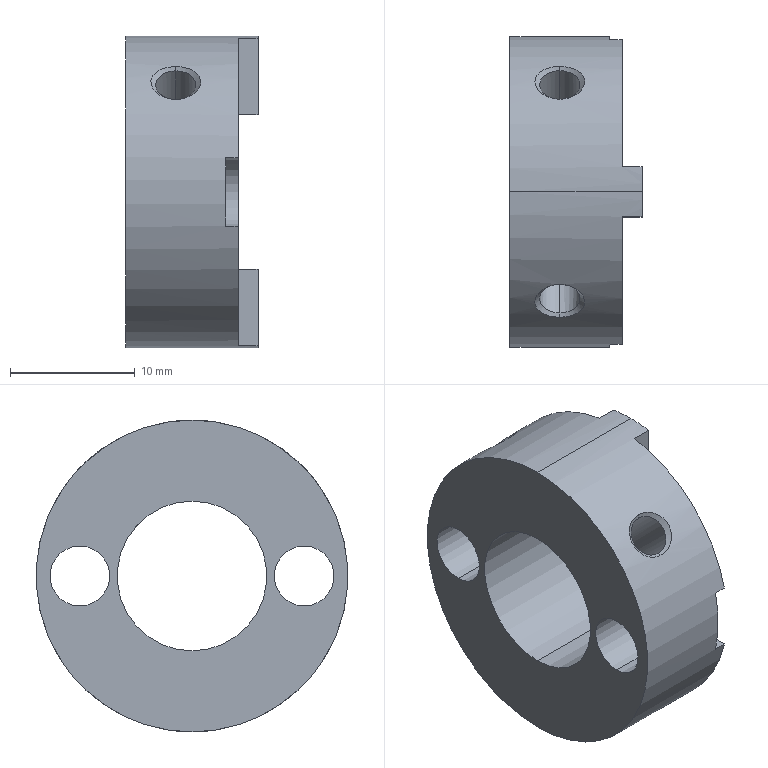Part | STEP file | _DBA11-D25-d10-e12-002.stp | 1 solid | 47 faces | box 10.6 x 25 x 25 mm | volume 2996 mm3 | cylinder 21 | plane 14 | cone 12 | commonest cylinder face diameters 2.013 x4 3.242 x4 4.8 x4 13 x3 5.58 x2 12 x2